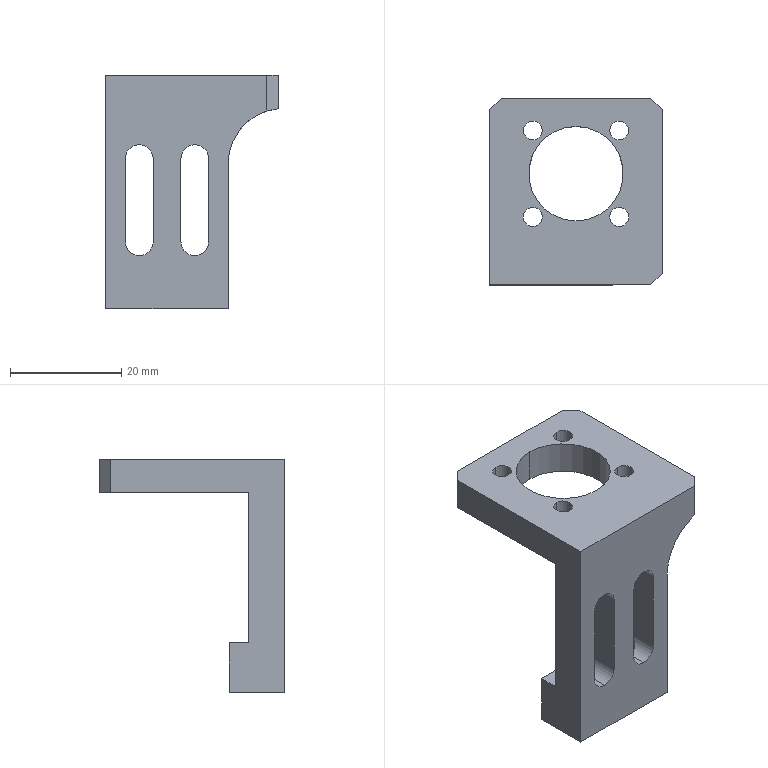NC program | NX | posted with a generic post | part box 31 x 33.478 x 42 mm
Whole program:
N10 G17 G21 G94 G90
(FLOOR_WALL_COPY , TOOL : D80)
N12 T19 M6
N14 G54
N16 G17 G0 G90 X-58.5 Y0. B0. C0. S6500 M3
N18 G43 Z30. H19
N20 Z5.
N22 G94 G1 Z2. F1500.
N24 X-55.5
N26 X55.5
N28 X58.5
N30 Z5.
N32 G0 Z30.
N34 X-58.5
N36 Z4.
N38 G1 Z1.
N40 X-55.5
N42 X55.5
N44 X58.5
N46 Z4.
N48 G0 Z30.
N50 X-58.5
N52 Z3.
N54 G1 Z0.
N56 X-55.5
N58 X55.5
N60 X58.5
N62 Z3.
N64 G0 Z30.
N66 M5
(DRILLING_COPY , TOOL : D6A45)
N68 T01 M6
N70 G54
N72 G17 G0 G90 X1.5 Y11.739 B0. C0. S9500 M3
N74 G43 Z30. H1
N76 G94 G81 G98 Z-1. F250. R3.
N78 X-10.5
N80 G80
N82 G0 X-10.5 Y11.739 Z30.
N84 M5
(DRILLING_COPY_COPY_COPY_1 , TOOL : 2.5ZT)
N86 T02 M6
N88 G54
N90 G17 G0 G90 X1.5 Y11.739 B0. C0. S2000 M3
N92 G43 Z30. H2
N94 G94 G83 G98 Z-13.011 F100. Q2. R3.
N96 X-10.5
N98 G80
N100 G0 X-10.5 Y11.739 Z30.
N102 M5
(PLANAR_MILL_COPY_COPY , TOOL : D6A45)
N104 T01 M6
N106 G54
N108 G17 G0 G90 X1.4 Y11.956 B0. C0. S9500 M3
N110 G43 Z30. H1
N112 Z0.5
N114 G94 G1 Z-1. F800.
N116 G3 X1.85 Y11.739 R0.5
N118 X1.5 Y12.089 R0.35 F1250.
N120 X1.85 Y11.739 R-0.35
N122 X1.4 Y11.522 R0.5
N124 G1 Z0.5
N126 G0 Z30.
N128 X-3.634 Y5.339
N130 Z0.5
N132 G1 Z-1. F800.
N134 G3 X-4.5 Y5.839 R1.
N136 G1 X-15.5 F1250.
N138 G2 X-16.4 Y6.739 R0.9
N140 G1 Y16.739
N142 G2 X-15.5 Y17.639 R0.9
N144 G1 X6.5
N146 G2 X7.4 Y16.739 R0.9
N148 G1 Y6.739
N150 G2 X6.5 Y5.839 R0.9
N152 G1 X-4.5
N154 G3 X-5.366 Y5.339 R1.
N156 G1 Z0.5
N158 G0 Z30.
N160 X-10.283 Y11.84
N162 Z0.5
N164 G1 Z-1. F800.
N166 G3 X-10.5 Y11.389 R0.5
N168 X-10.15 Y11.739 R0.35 F1250.
N170 X-10.5 Y11.389 R-0.35
N172 X-10.717 Y11.84 R0.5
N174 G1 Z0.5
N176 G0 Z30.
N178 M5
N180 M2